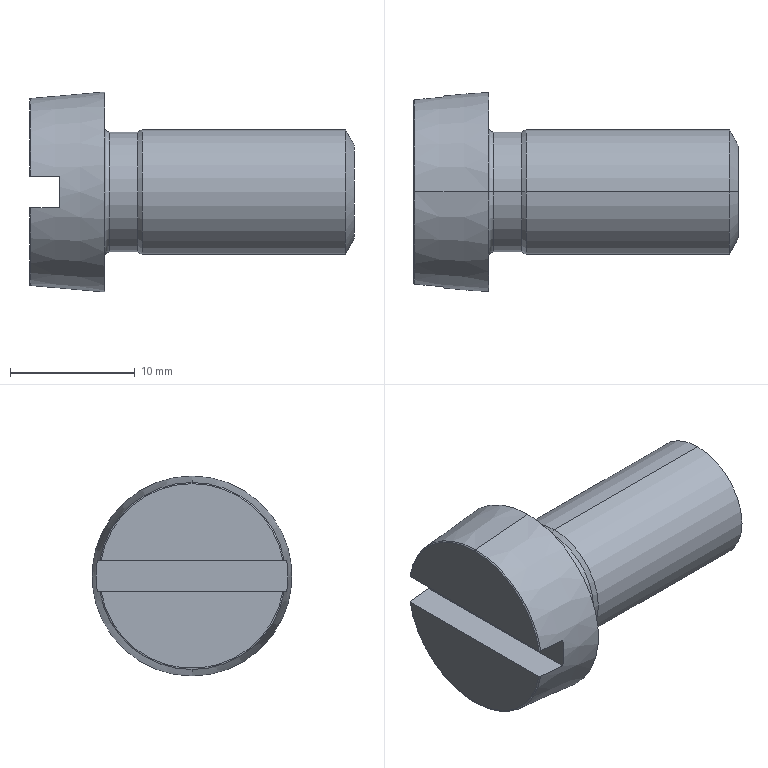Part | SolidWorks | features Cut 1, LPattern 1, RevCut 1, Revolution 1 | 1 solid | 22 faces | box 26 x 16 x 16 mm | volume 2579 mm3 | plane 7 | cone 6 | torus 5 | cylinder 4 | commonest cylinder face diameters 9.6 x2 10 x2
STEP:
#1=CARTESIAN_POINT('',(26.,0.,3.701));
#2=VERTEX_POINT('',#1);
#3=CARTESIAN_POINT('',(26.,0.,-3.701));
#4=VERTEX_POINT('',#3);
#5=CARTESIAN_POINT('',(26.,0.,0.));
#6=DIRECTION('',(-1.,0.,0.));
#7=DIRECTION('',(0.,0.,1.));
#8=AXIS2_PLACEMENT_3D('',#5,#6,#7);
#9=CIRCLE('',#8,3.701);
#10=EDGE_CURVE('',#2,#4,#9,.T.);
#11=ORIENTED_EDGE('',*,*,#10,.T.);
#12=CARTESIAN_POINT('',(25.25,0.,-5.));
#13=VERTEX_POINT('',#12);
#14=CARTESIAN_POINT('',(25.25,0.,-5.));
#15=DIRECTION('',(-0.5,0.,-0.866));
#16=VECTOR('',#15,1000.);
#17=LINE('',#14,#16);
#18=EDGE_CURVE('',#4,#13,#17,.T.);
#19=ORIENTED_EDGE('',*,*,#18,.T.);
#20=CARTESIAN_POINT('',(25.25,0.,5.));
#21=VERTEX_POINT('',#20);
#22=CARTESIAN_POINT('',(25.25,0.,0.));
#23=DIRECTION('',(-1.,0.,0.));
#24=DIRECTION('',(0.,0.,1.));
#25=AXIS2_PLACEMENT_3D('',#22,#23,#24);
#26=CIRCLE('',#25,5.);
#27=EDGE_CURVE('',#21,#13,#26,.T.);
#28=ORIENTED_EDGE('',*,*,#27,.F.);
#29=CARTESIAN_POINT('',(25.25,0.,5.));
#30=DIRECTION('',(-0.5,0.,0.866));
#31=VECTOR('',#30,1000.);
#32=LINE('',#29,#31);
#33=EDGE_CURVE('',#2,#21,#32,.T.);
#34=ORIENTED_EDGE('',*,*,#33,.F.);
#35=EDGE_LOOP('',(#11,#19,#28,#34));
#36=FACE_OUTER_BOUND('',#35,.T.);
#37=CARTESIAN_POINT('',(25.25,0.,0.));
#38=DIRECTION('',(-1.,0.,0.));
#39=DIRECTION('',(0.,0.,1.));
#40=AXIS2_PLACEMENT_3D('',#37,#38,#39);
#41=CONICAL_SURFACE('',#40,5.,1.047);
#42=ADVANCED_FACE('',(#36),#41,.T.);
#43=CARTESIAN_POINT('',(8.654,0.,4.8));
#44=VERTEX_POINT('',#43);
#45=CARTESIAN_POINT('',(8.654,0.,-4.8));
#46=VERTEX_POINT('',#45);
#47=CARTESIAN_POINT('',(8.654,0.,0.));
#48=DIRECTION('',(-1.,0.,0.));
#49=DIRECTION('',(0.,0.,1.));
#50=AXIS2_PLACEMENT_3D('',#47,#48,#49);
#51=CIRCLE('',#50,4.8);
#52=EDGE_CURVE('',#44,#46,#51,.T.);
#53=ORIENTED_EDGE('',*,*,#52,.F.);
#54=CARTESIAN_POINT('',(9.,0.,5.));
#55=VERTEX_POINT('',#54);
#56=CARTESIAN_POINT('',(9.,0.,5.));
#57=DIRECTION('',(0.866,0.,0.5));
#58=VECTOR('',#57,1000.);
#59=LINE('',#56,#58);
#60=EDGE_CURVE('',#44,#55,#59,.T.);
#61=ORIENTED_EDGE('',*,*,#60,.T.);
#62=CARTESIAN_POINT('',(9.,0.,-5.));
#63=VERTEX_POINT('',#62);
#64=CARTESIAN_POINT('',(9.,0.,0.));
#65=DIRECTION('',(-1.,0.,0.));
#66=DIRECTION('',(0.,0.,1.));
#67=AXIS2_PLACEMENT_3D('',#64,#65,#66);
#68=CIRCLE('',#67,5.);
#69=EDGE_CURVE('',#55,#63,#68,.T.);
#70=ORIENTED_EDGE('',*,*,#69,.T.);
#71=CARTESIAN_POINT('',(9.,0.,-5.));
#72=DIRECTION('',(0.866,0.,-0.5));
#73=VECTOR('',#72,1000.);
#74=LINE('',#71,#73);
#75=EDGE_CURVE('',#46,#63,#74,.T.);
#76=ORIENTED_EDGE('',*,*,#75,.F.);
#77=EDGE_LOOP('',(#53,#61,#70,#76));
#78=FACE_OUTER_BOUND('',#77,.T.);
#79=CARTESIAN_POINT('',(9.,0.,0.));
#80=DIRECTION('',(1.,0.,0.));
#81=DIRECTION('',(0.,0.,-1.));
#82=AXIS2_PLACEMENT_3D('',#79,#80,#81);
#83=CONICAL_SURFACE('',#82,5.,0.5236);
#84=ADVANCED_FACE('',(#78),#83,.T.);
#85=ORIENTED_EDGE('',*,*,#52,.T.);
#86=CARTESIAN_POINT('',(6.4,0.,-4.8));
#87=VERTEX_POINT('',#86);
#88=CARTESIAN_POINT('',(0.,0.,-4.8));
#89=DIRECTION('',(-1.,0.,0.));
#90=VECTOR('',#89,1000.);
#91=LINE('',#88,#90);
#92=EDGE_CURVE('',#46,#87,#91,.T.);
#93=ORIENTED_EDGE('',*,*,#92,.T.);
#94=CARTESIAN_POINT('',(6.4,0.,4.8));
#95=VERTEX_POINT('',#94);
#96=CARTESIAN_POINT('',(6.4,0.,0.));
#97=DIRECTION('',(-1.,0.,0.));
#98=DIRECTION('',(0.,0.,1.));
#99=AXIS2_PLACEMENT_3D('',#96,#97,#98);
#100=CIRCLE('',#99,4.8);
#101=EDGE_CURVE('',#95,#87,#100,.T.);
#102=ORIENTED_EDGE('',*,*,#101,.F.);
#103=CARTESIAN_POINT('',(0.,0.,4.8));
#104=DIRECTION('',(-1.,0.,0.));
#105=VECTOR('',#104,1000.);
#106=LINE('',#103,#105);
#107=EDGE_CURVE('',#44,#95,#106,.T.);
#108=ORIENTED_EDGE('',*,*,#107,.F.);
#109=EDGE_LOOP('',(#85,#93,#102,#108));
#110=FACE_OUTER_BOUND('',#109,.T.);
#111=CARTESIAN_POINT('',(0.,0.,0.));
#112=DIRECTION('',(-1.,0.,0.));
#113=DIRECTION('',(0.,0.,1.));
#114=AXIS2_PLACEMENT_3D('',#111,#112,#113);
#115=CYLINDRICAL_SURFACE('',#114,4.8);
#116=ADVANCED_FACE('',(#110),#115,.T.);
#117=CARTESIAN_POINT('',(6.,0.,-5.2));
#118=VERTEX_POINT('',#117);
#119=CARTESIAN_POINT('',(6.,0.,5.2));
#120=VERTEX_POINT('',#119);
#121=CARTESIAN_POINT('',(6.,0.,0.));
#122=DIRECTION('',(-1.,0.,0.));
#123=DIRECTION('',(0.,0.,1.));
#124=AXIS2_PLACEMENT_3D('',#121,#122,#123);
#125=CIRCLE('',#124,5.2);
#126=EDGE_CURVE('',#118,#120,#125,.T.);
#127=ORIENTED_EDGE('',*,*,#126,.F.);
#128=CARTESIAN_POINT('',(6.4,0.,-5.2));
#129=DIRECTION('',(0.,1.,0.));
#130=DIRECTION('',(0.,0.,1.));
#131=AXIS2_PLACEMENT_3D('',#128,#129,#130);
#132=CIRCLE('',#131,0.4);
#133=EDGE_CURVE('',#118,#87,#132,.T.);
#134=ORIENTED_EDGE('',*,*,#133,.T.);
#135=CARTESIAN_POINT('',(6.4,0.,0.));
#136=DIRECTION('',(-1.,0.,0.));
#137=DIRECTION('',(0.,0.,1.));
#138=AXIS2_PLACEMENT_3D('',#135,#136,#137);
#139=CIRCLE('',#138,4.8);
#140=EDGE_CURVE('',#87,#95,#139,.T.);
#141=ORIENTED_EDGE('',*,*,#140,.T.);
#142=CARTESIAN_POINT('',(6.4,0.,5.2));
#143=DIRECTION('',(0.,-1.,0.));
#144=DIRECTION('',(0.,0.,-1.));
#145=AXIS2_PLACEMENT_3D('',#142,#143,#144);
#146=CIRCLE('',#145,0.4);
#147=EDGE_CURVE('',#120,#95,#146,.T.);
#148=ORIENTED_EDGE('',*,*,#147,.F.);
#149=EDGE_LOOP('',(#127,#134,#141,#148));
#150=FACE_OUTER_BOUND('',#149,.T.);
#151=CARTESIAN_POINT('',(6.4,0.,0.));
#152=DIRECTION('',(-1.,0.,0.));
#153=DIRECTION('',(0.,0.,1.));
#154=AXIS2_PLACEMENT_3D('',#151,#152,#153);
#155=TOROIDAL_SURFACE('',#154,5.2,0.4);
#156=ADVANCED_FACE('',(#150),#155,.F.);
#157=CARTESIAN_POINT('',(0.09128,0.,7.483));
#158=VERTEX_POINT('',#157);
#159=CARTESIAN_POINT('',(0.09128,7.378,1.25));
#160=VERTEX_POINT('',#159);
#161=CARTESIAN_POINT('',(0.09128,0.,0.));
#162=DIRECTION('',(-1.,0.,0.));
#163=DIRECTION('',(0.,0.,1.));
#164=AXIS2_PLACEMENT_3D('',#161,#162,#163);
#165=CIRCLE('',#164,7.483);
#166=EDGE_CURVE('',#158,#160,#165,.T.);
#167=ORIENTED_EDGE('',*,*,#166,.F.);
#168=CARTESIAN_POINT('',(6.,0.,8.));
#169=VERTEX_POINT('',#168);
#170=CARTESIAN_POINT('',(6.,0.,8.));
#171=DIRECTION('',(0.9962,0.,0.08716));
#172=VECTOR('',#171,1000.);
#173=LINE('',#170,#172);
#174=EDGE_CURVE('',#158,#169,#173,.T.);
#175=ORIENTED_EDGE('',*,*,#174,.T.);
#176=CARTESIAN_POINT('',(6.,0.,-8.));
#177=VERTEX_POINT('',#176);
#178=CARTESIAN_POINT('',(6.,0.,0.));
#179=DIRECTION('',(-1.,0.,0.));
#180=DIRECTION('',(0.,0.,1.));
#181=AXIS2_PLACEMENT_3D('',#178,#179,#180);
#182=CIRCLE('',#181,8.);
#183=EDGE_CURVE('',#169,#177,#182,.T.);
#184=ORIENTED_EDGE('',*,*,#183,.T.);
#185=CARTESIAN_POINT('',(0.09128,0.,-7.483));
#186=VERTEX_POINT('',#185);
#187=CARTESIAN_POINT('',(6.,0.,-8.));
#188=DIRECTION('',(0.9962,0.,-0.08716));
#189=VECTOR('',#188,1000.);
#190=LINE('',#187,#189);
#191=EDGE_CURVE('',#186,#177,#190,.T.);
#192=ORIENTED_EDGE('',*,*,#191,.F.);
#193=CARTESIAN_POINT('',(0.09128,7.378,-1.25));
#194=VERTEX_POINT('',#193);
#195=CARTESIAN_POINT('',(0.09128,0.,0.));
#196=DIRECTION('',(-1.,0.,0.));
#197=DIRECTION('',(0.,0.,1.));
#198=AXIS2_PLACEMENT_3D('',#195,#196,#197);
#199=CIRCLE('',#198,7.483);
#200=EDGE_CURVE('',#194,#186,#199,.T.);
#201=ORIENTED_EDGE('',*,*,#200,.F.);
#202=CARTESIAN_POINT('',(2.4,7.583,-1.25));
#203=VERTEX_POINT('',#202);
#204=CARTESIAN_POINT('',(0.09128,7.378,-1.25));
#205=CARTESIAN_POINT('',(0.4301,7.408,-1.25));
#206=CARTESIAN_POINT('',(0.769,7.438,-1.25));
#207=CARTESIAN_POINT('',(1.108,7.468,-1.25));
#208=CARTESIAN_POINT('',(1.539,7.506,-1.25));
#209=CARTESIAN_POINT('',(1.969,7.545,-1.25));
#210=CARTESIAN_POINT('',(2.4,7.583,-1.25));
#211=B_SPLINE_CURVE_WITH_KNOTS('',3,(#204,#205,#206,#207,#208,#209,#210),.UNSPECIFIED.,.F.,.F.,(4,3,4),(0.01291,0.01393,0.01523),.UNSPECIFIED.);
#212=EDGE_CURVE('',#194,#203,#211,.T.);
#213=ORIENTED_EDGE('',*,*,#212,.T.);
#214=CARTESIAN_POINT('',(2.4,7.583,1.25));
#215=VERTEX_POINT('',#214);
#216=CARTESIAN_POINT('',(2.4,0.,0.));
#217=DIRECTION('',(-1.,0.,0.));
#218=DIRECTION('',(0.,-1.,0.));
#219=AXIS2_PLACEMENT_3D('',#216,#217,#218);
#220=CIRCLE('',#219,7.685);
#221=EDGE_CURVE('',#215,#203,#220,.T.);
#222=ORIENTED_EDGE('',*,*,#221,.F.);
#223=CARTESIAN_POINT('',(2.4,7.583,1.25));
#224=CARTESIAN_POINT('',(1.969,7.545,1.25));
#225=CARTESIAN_POINT('',(1.539,7.506,1.25));
#226=CARTESIAN_POINT('',(1.108,7.468,1.25));
#227=CARTESIAN_POINT('',(0.769,7.438,1.25));
#228=CARTESIAN_POINT('',(0.4301,7.408,1.25));
#229=CARTESIAN_POINT('',(0.09128,7.378,1.25));
#230=B_SPLINE_CURVE_WITH_KNOTS('',3,(#223,#224,#225,#226,#227,#228,#229),.UNSPECIFIED.,.F.,.F.,(4,3,4),(0.01263,0.01393,0.01495),.UNSPECIFIED.);
#231=EDGE_CURVE('',#215,#160,#230,.T.);
#232=ORIENTED_EDGE('',*,*,#231,.T.);
#233=EDGE_LOOP('',(#167,#175,#184,#192,#201,#213,#222,#232));
#234=FACE_OUTER_BOUND('',#233,.T.);
#235=CARTESIAN_POINT('',(6.,0.,0.));
#236=DIRECTION('',(1.,0.,0.));
#237=DIRECTION('',(0.,0.,-1.));
#238=AXIS2_PLACEMENT_3D('',#235,#236,#237);
#239=CONICAL_SURFACE('',#238,8.,0.08727);
#240=ADVANCED_FACE('',(#234),#239,.T.);
#241=CARTESIAN_POINT('',(0.09128,-7.378,1.25));
#242=VERTEX_POINT('',#241);
#243=CARTESIAN_POINT('',(0.09128,0.,0.));
#244=DIRECTION('',(-1.,0.,0.));
#245=DIRECTION('',(0.,0.,1.));
#246=AXIS2_PLACEMENT_3D('',#243,#244,#245);
#247=CIRCLE('',#246,7.483);
#248=EDGE_CURVE('',#242,#158,#247,.T.);
#249=ORIENTED_EDGE('',*,*,#248,.T.);
#250=CARTESIAN_POINT('',(0.,0.,7.383));
#251=VERTEX_POINT('',#250);
#252=CARTESIAN_POINT('',(0.1,0.,7.383));
#253=DIRECTION('',(0.,-1.,0.));
#254=DIRECTION('',(0.,0.,-1.));
#255=AXIS2_PLACEMENT_3D('',#252,#253,#254);
#256=CIRCLE('',#255,0.1);
#257=EDGE_CURVE('',#158,#251,#256,.T.);
#258=ORIENTED_EDGE('',*,*,#257,.T.);
#259=CARTESIAN_POINT('',(0.,-7.277,1.25));
#260=VERTEX_POINT('',#259);
#261=CARTESIAN_POINT('',(0.,0.,0.));
#262=DIRECTION('',(-1.,0.,0.));
#263=DIRECTION('',(0.,0.,1.));
#264=AXIS2_PLACEMENT_3D('',#261,#262,#263);
#265=CIRCLE('',#264,7.383);
#266=EDGE_CURVE('',#260,#251,#265,.T.);
#267=ORIENTED_EDGE('',*,*,#266,.F.);
#268=CARTESIAN_POINT('',(0.,-7.277,1.25));
#269=CARTESIAN_POINT('',(0.,-7.286,1.25));
#270=CARTESIAN_POINT('',(0.001125,-7.294,1.25));
#271=CARTESIAN_POINT('',(0.003323,-7.303,1.25));
#272=CARTESIAN_POINT('',(0.006228,-7.314,1.25));
#273=CARTESIAN_POINT('',(0.0111,-7.325,1.25));
#274=CARTESIAN_POINT('',(0.01756,-7.334,1.25));
#275=CARTESIAN_POINT('',(0.0217,-7.34,1.25));
#276=CARTESIAN_POINT('',(0.02655,-7.346,1.25));
#277=CARTESIAN_POINT('',(0.03193,-7.351,1.25));
#278=CARTESIAN_POINT('',(0.04004,-7.359,1.25));
#279=CARTESIAN_POINT('',(0.04957,-7.365,1.25));
#280=CARTESIAN_POINT('',(0.05975,-7.37,1.25));
#281=CARTESIAN_POINT('',(0.06967,-7.374,1.25));
#282=CARTESIAN_POINT('',(0.08047,-7.377,1.25));
#283=CARTESIAN_POINT('',(0.09128,-7.378,1.25));
#284=B_SPLINE_CURVE_WITH_KNOTS('',3,(#268,#269,#270,#271,#272,#273,#274,#275,#276,#277,#278,#279,#280,#281,#282,#283),.UNSPECIFIED.,.F.,.F.,(4,3,3,3,3,4),(0.0005472,0.0005733,0.0006079,0.0006299,0.0006633,0.0006959),.UNSPECIFIED.);
#285=EDGE_CURVE('',#260,#242,#284,.T.);
#286=ORIENTED_EDGE('',*,*,#285,.T.);
#287=EDGE_LOOP('',(#249,#258,#267,#286));
#288=FACE_OUTER_BOUND('',#287,.T.);
#289=CARTESIAN_POINT('',(0.1,0.,0.));
#290=DIRECTION('',(-1.,0.,0.));
#291=DIRECTION('',(0.,0.,1.));
#292=AXIS2_PLACEMENT_3D('',#289,#290,#291);
#293=TOROIDAL_SURFACE('',#292,7.383,0.1);
#294=ADVANCED_FACE('',(#288),#293,.T.);
#295=ORIENTED_EDGE('',*,*,#27,.T.);
#296=CARTESIAN_POINT('',(0.,0.,-5.));
#297=DIRECTION('',(-1.,0.,0.));
#298=VECTOR('',#297,1000.);
#299=LINE('',#296,#298);
#300=EDGE_CURVE('',#13,#63,#299,.T.);
#301=ORIENTED_EDGE('',*,*,#300,.T.);
#302=ORIENTED_EDGE('',*,*,#69,.F.);
#303=CARTESIAN_POINT('',(0.,0.,5.));
#304=DIRECTION('',(-1.,0.,0.));
#305=VECTOR('',#304,1000.);
#306=LINE('',#303,#305);
#307=EDGE_CURVE('',#21,#55,#306,.T.);
#308=ORIENTED_EDGE('',*,*,#307,.F.);
#309=EDGE_LOOP('',(#295,#301,#302,#308));
#310=FACE_OUTER_BOUND('',#309,.T.);
#311=CARTESIAN_POINT('',(0.,0.,0.));
#312=DIRECTION('',(-1.,0.,0.));
#313=DIRECTION('',(0.,0.,1.));
#314=AXIS2_PLACEMENT_3D('',#311,#312,#313);
#315=CYLINDRICAL_SURFACE('',#314,5.);
#316=ADVANCED_FACE('',(#310),#315,.T.);
#317=ORIENTED_EDGE('',*,*,#300,.F.);
#318=CARTESIAN_POINT('',(25.25,0.,0.));
#319=DIRECTION('',(-1.,0.,0.));
#320=DIRECTION('',(0.,0.,1.));
#321=AXIS2_PLACEMENT_3D('',#318,#319,#320);
#322=CIRCLE('',#321,5.);
#323=EDGE_CURVE('',#13,#21,#322,.T.);
#324=ORIENTED_EDGE('',*,*,#323,.T.);
#325=ORIENTED_EDGE('',*,*,#307,.T.);
#326=CARTESIAN_POINT('',(9.,0.,0.));
#327=DIRECTION('',(-1.,0.,0.));
#328=DIRECTION('',(0.,0.,1.));
#329=AXIS2_PLACEMENT_3D('',#326,#327,#328);
#330=CIRCLE('',#329,5.);
#331=EDGE_CURVE('',#63,#55,#330,.T.);
#332=ORIENTED_EDGE('',*,*,#331,.F.);
#333=EDGE_LOOP('',(#317,#324,#325,#332));
#334=FACE_OUTER_BOUND('',#333,.T.);
#335=CARTESIAN_POINT('',(0.,0.,0.));
#336=DIRECTION('',(-1.,0.,0.));
#337=DIRECTION('',(0.,0.,1.));
#338=AXIS2_PLACEMENT_3D('',#335,#336,#337);
#339=CYLINDRICAL_SURFACE('',#338,5.);
#340=ADVANCED_FACE('',(#334),#339,.T.);
#341=ORIENTED_EDGE('',*,*,#266,.T.);
#342=CARTESIAN_POINT('',(0.,7.277,1.25));
#343=VERTEX_POINT('',#342);
#344=CARTESIAN_POINT('',(0.,0.,0.));
#345=DIRECTION('',(-1.,0.,0.));
#346=DIRECTION('',(0.,0.,1.));
#347=AXIS2_PLACEMENT_3D('',#344,#345,#346);
#348=CIRCLE('',#347,7.383);
#349=EDGE_CURVE('',#251,#343,#348,.T.);
#350=ORIENTED_EDGE('',*,*,#349,.T.);
#351=CARTESIAN_POINT('',(0.,7.902,1.25));
#352=DIRECTION('',(0.,1.,0.));
#353=VECTOR('',#352,1000.);
#354=LINE('',#351,#353);
#355=EDGE_CURVE('',#260,#343,#354,.T.);
#356=ORIENTED_EDGE('',*,*,#355,.F.);
#357=EDGE_LOOP('',(#341,#350,#356));
#358=FACE_OUTER_BOUND('',#357,.T.);
#359=CARTESIAN_POINT('',(0.,0.,0.));
#360=DIRECTION('',(1.,0.,0.));
#361=DIRECTION('',(0.,0.,-1.));
#362=AXIS2_PLACEMENT_3D('',#359,#360,#361);
#363=PLANE('',#362);
#364=ADVANCED_FACE('',(#358),#363,.F.);
#365=ORIENTED_EDGE('',*,*,#257,.F.);
#366=ORIENTED_EDGE('',*,*,#166,.T.);
#367=CARTESIAN_POINT('',(0.09128,7.378,1.25));
#368=CARTESIAN_POINT('',(0.08575,7.377,1.25));
#369=CARTESIAN_POINT('',(0.08023,7.376,1.25));
#370=CARTESIAN_POINT('',(0.07485,7.375,1.25));
#371=CARTESIAN_POINT('',(0.06418,7.372,1.25));
#372=CARTESIAN_POINT('',(0.05384,7.368,1.25));
#373=CARTESIAN_POINT('',(0.04468,7.361,1.25));
#374=CARTESIAN_POINT('',(0.03547,7.355,1.25));
#375=CARTESIAN_POINT('',(0.02719,7.347,1.25));
#376=CARTESIAN_POINT('',(0.02051,7.338,1.25));
#377=CARTESIAN_POINT('',(0.01375,7.329,1.25));
#378=CARTESIAN_POINT('',(0.008429,7.319,1.25));
#379=CARTESIAN_POINT('',(0.00497,7.308,1.25));
#380=CARTESIAN_POINT('',(0.001695,7.298,1.25));
#381=CARTESIAN_POINT('',(0.,7.288,1.25));
#382=CARTESIAN_POINT('',(0.,7.277,1.25));
#383=B_SPLINE_CURVE_WITH_KNOTS('',3,(#367,#368,#369,#370,#371,#372,#373,#374,#375,#376,#377,#378,#379,#380,#381,#382),.UNSPECIFIED.,.F.,.F.,(4,3,3,3,3,4),(0.0003879,0.0004045,0.0004376,0.0004709,0.0005047,0.0005367),.UNSPECIFIED.);
#384=EDGE_CURVE('',#160,#343,#383,.T.);
#385=ORIENTED_EDGE('',*,*,#384,.T.);
#386=ORIENTED_EDGE('',*,*,#349,.F.);
#387=EDGE_LOOP('',(#365,#366,#385,#386));
#388=FACE_OUTER_BOUND('',#387,.T.);
#389=CARTESIAN_POINT('',(0.1,0.,0.));
#390=DIRECTION('',(-1.,0.,0.));
#391=DIRECTION('',(0.,0.,1.));
#392=AXIS2_PLACEMENT_3D('',#389,#390,#391);
#393=TOROIDAL_SURFACE('',#392,7.383,0.1);
#394=ADVANCED_FACE('',(#388),#393,.T.);
#395=CARTESIAN_POINT('',(0.,7.277,-1.25));
#396=VERTEX_POINT('',#395);
#397=CARTESIAN_POINT('',(0.,-7.277,-1.25));
#398=VERTEX_POINT('',#397);
#399=CARTESIAN_POINT('',(0.,0.,0.));
#400=DIRECTION('',(-1.,0.,0.));
#401=DIRECTION('',(0.,0.,1.));
#402=AXIS2_PLACEMENT_3D('',#399,#400,#401);
#403=CIRCLE('',#402,7.383);
#404=EDGE_CURVE('',#396,#398,#403,.T.);
#405=ORIENTED_EDGE('',*,*,#404,.T.);
#406=CARTESIAN_POINT('',(0.,7.902,-1.25));
#407=DIRECTION('',(0.,-1.,0.));
#408=VECTOR('',#407,1000.);
#409=LINE('',#406,#408);
#410=EDGE_CURVE('',#396,#398,#409,.T.);
#411=ORIENTED_EDGE('',*,*,#410,.F.);
#412=EDGE_LOOP('',(#405,#411));
#413=FACE_OUTER_BOUND('',#412,.T.);
#414=CARTESIAN_POINT('',(0.,0.,0.));
#415=DIRECTION('',(1.,0.,0.));
#416=DIRECTION('',(0.,0.,-1.));
#417=AXIS2_PLACEMENT_3D('',#414,#415,#416);
#418=PLANE('',#417);
#419=ADVANCED_FACE('',(#413),#418,.F.);
#420=ORIENTED_EDGE('',*,*,#200,.T.);
#421=CARTESIAN_POINT('',(0.09128,-7.378,-1.25));
#422=VERTEX_POINT('',#421);
#423=CARTESIAN_POINT('',(0.09128,0.,0.));
#424=DIRECTION('',(-1.,0.,0.));
#425=DIRECTION('',(0.,0.,1.));
#426=AXIS2_PLACEMENT_3D('',#423,#424,#425);
#427=CIRCLE('',#426,7.483);
#428=EDGE_CURVE('',#186,#422,#427,.T.);
#429=ORIENTED_EDGE('',*,*,#428,.T.);
#430=CARTESIAN_POINT('',(0.09128,-7.378,-1.25));
#431=CARTESIAN_POINT('',(0.08699,-7.378,-1.25));
#432=CARTESIAN_POINT('',(0.08271,-7.377,-1.25));
#433=CARTESIAN_POINT('',(0.07851,-7.376,-1.25));
#434=CARTESIAN_POINT('',(0.06773,-7.374,-1.25));
#435=CARTESIAN_POINT('',(0.05723,-7.369,-1.25));
#436=CARTESIAN_POINT('',(0.04784,-7.363,-1.25));
#437=CARTESIAN_POINT('',(0.04216,-7.36,-1.25));
#438=CARTESIAN_POINT('',(0.0368,-7.356,-1.25));
#439=CARTESIAN_POINT('',(0.03193,-7.351,-1.25));
#440=CARTESIAN_POINT('',(0.02366,-7.343,-1.25));
#441=CARTESIAN_POINT('',(0.01663,-7.334,-1.25));
#442=CARTESIAN_POINT('',(0.01141,-7.324,-1.25));
#443=CARTESIAN_POINT('',(0.006197,-7.314,-1.25));
#444=CARTESIAN_POINT('',(0.002648,-7.303,-1.25));
#445=CARTESIAN_POINT('',(0.001037,-7.291,-1.25));
#446=CARTESIAN_POINT('',(0.0003474,-7.287,-1.25));
#447=CARTESIAN_POINT('',(0.,-7.282,-1.25));
#448=CARTESIAN_POINT('',(0.,-7.277,-1.25));
#449=B_SPLINE_CURVE_WITH_KNOTS('',3,(#430,#431,#432,#433,#434,#435,#436,#437,#438,#439,#440,#441,#442,#443,#444,#445,#446,#447,#448),.UNSPECIFIED.,.F.,.F.,(4,3,3,3,3,3,4),(0.0005639,0.0005767,0.0006098,0.0006297,0.0006638,0.0006979,0.0007125),.UNSPECIFIED.);
#450=EDGE_CURVE('',#422,#398,#449,.T.);
#451=ORIENTED_EDGE('',*,*,#450,.T.);
#452=ORIENTED_EDGE('',*,*,#404,.F.);
#453=CARTESIAN_POINT('',(0.,7.277,-1.25));
#454=CARTESIAN_POINT('',(0.,7.28,-1.25));
#455=CARTESIAN_POINT('',(0.0001312,7.283,-1.25));
#456=CARTESIAN_POINT('',(0.0003928,7.286,-1.25));
#457=CARTESIAN_POINT('',(0.001398,7.297,-1.25));
#458=CARTESIAN_POINT('',(0.004397,7.309,-1.25));
#459=CARTESIAN_POINT('',(0.009153,7.319,-1.25));
#460=CARTESIAN_POINT('',(0.0139,7.33,-1.25));
#461=CARTESIAN_POINT('',(0.02052,7.34,-1.25));
#462=CARTESIAN_POINT('',(0.0285,7.348,-1.25));
#463=CARTESIAN_POINT('',(0.03638,7.356,-1.25));
#464=CARTESIAN_POINT('',(0.0458,7.363,-1.25));
#465=CARTESIAN_POINT('',(0.05598,7.368,-1.25));
#466=CARTESIAN_POINT('',(0.06601,7.373,-1.25));
#467=CARTESIAN_POINT('',(0.07705,7.376,-1.25));
#468=CARTESIAN_POINT('',(0.08817,7.378,-1.25));
#469=CARTESIAN_POINT('',(0.08921,7.378,-1.25));
#470=CARTESIAN_POINT('',(0.09025,7.378,-1.25));
#471=CARTESIAN_POINT('',(0.09128,7.378,-1.25));
#472=B_SPLINE_CURVE_WITH_KNOTS('',3,(#453,#454,#455,#456,#457,#458,#459,#460,#461,#462,#463,#464,#465,#466,#467,#468,#469,#470,#471),.UNSPECIFIED.,.F.,.F.,(4,3,3,3,3,3,4),(0.00009337,0.0001023,0.0001368,0.0001713,0.0002054,0.000239,0.0002421),.UNSPECIFIED.);
#473=EDGE_CURVE('',#396,#194,#472,.T.);
#474=ORIENTED_EDGE('',*,*,#473,.T.);
#475=EDGE_LOOP('',(#420,#429,#451,#452,#474));
#476=FACE_OUTER_BOUND('',#475,.T.);
#477=CARTESIAN_POINT('',(0.1,0.,0.));
#478=DIRECTION('',(-1.,0.,0.));
#479=DIRECTION('',(0.,0.,1.));
#480=AXIS2_PLACEMENT_3D('',#477,#478,#479);
#481=TOROIDAL_SURFACE('',#480,7.383,0.1);
#482=ADVANCED_FACE('',(#476),#481,.T.);
#483=ORIENTED_EDGE('',*,*,#174,.F.);
#484=ORIENTED_EDGE('',*,*,#248,.F.);
#485=CARTESIAN_POINT('',(2.4,-7.583,1.25));
#486=VERTEX_POINT('',#485);
#487=CARTESIAN_POINT('',(0.09128,-7.378,1.25));
#488=CARTESIAN_POINT('',(0.4301,-7.408,1.25));
#489=CARTESIAN_POINT('',(0.769,-7.438,1.25));
#490=CARTESIAN_POINT('',(1.108,-7.468,1.25));
#491=CARTESIAN_POINT('',(1.539,-7.506,1.25));
#492=CARTESIAN_POINT('',(1.969,-7.545,1.25));
#493=CARTESIAN_POINT('',(2.4,-7.583,1.25));
#494=B_SPLINE_CURVE_WITH_KNOTS('',3,(#487,#488,#489,#490,#491,#492,#493),.UNSPECIFIED.,.F.,.F.,(4,3,4),(0.01291,0.01393,0.01523),.UNSPECIFIED.);
#495=EDGE_CURVE('',#242,#486,#494,.T.);
#496=ORIENTED_EDGE('',*,*,#495,.T.);
#497=CARTESIAN_POINT('',(2.4,-7.583,-1.25));
#498=VERTEX_POINT('',#497);
#499=CARTESIAN_POINT('',(2.4,0.,0.));
#500=DIRECTION('',(-1.,0.,0.));
#501=DIRECTION('',(0.,-1.,0.));
#502=AXIS2_PLACEMENT_3D('',#499,#500,#501);
#503=CIRCLE('',#502,7.685);
#504=EDGE_CURVE('',#498,#486,#503,.T.);
#505=ORIENTED_EDGE('',*,*,#504,.F.);
#506=CARTESIAN_POINT('',(2.4,-7.583,-1.25));
#507=CARTESIAN_POINT('',(1.969,-7.545,-1.25));
#508=CARTESIAN_POINT('',(1.539,-7.506,-1.25));
#509=CARTESIAN_POINT('',(1.108,-7.468,-1.25));
#510=CARTESIAN_POINT('',(0.769,-7.438,-1.25));
#511=CARTESIAN_POINT('',(0.4301,-7.408,-1.25));
#512=CARTESIAN_POINT('',(0.09128,-7.378,-1.25));
#513=B_SPLINE_CURVE_WITH_KNOTS('',3,(#506,#507,#508,#509,#510,#511,#512),.UNSPECIFIED.,.F.,.F.,(4,3,4),(0.01263,0.01393,0.01495),.UNSPECIFIED.);
#514=EDGE_CURVE('',#498,#422,#513,.T.);
#515=ORIENTED_EDGE('',*,*,#514,.T.);
#516=ORIENTED_EDGE('',*,*,#428,.F.);
#517=ORIENTED_EDGE('',*,*,#191,.T.);
#518=CARTESIAN_POINT('',(6.,0.,0.));
#519=DIRECTION('',(-1.,0.,0.));
#520=DIRECTION('',(0.,0.,1.));
#521=AXIS2_PLACEMENT_3D('',#518,#519,#520);
#522=CIRCLE('',#521,8.);
#523=EDGE_CURVE('',#177,#169,#522,.T.);
#524=ORIENTED_EDGE('',*,*,#523,.T.);
#525=EDGE_LOOP('',(#483,#484,#496,#505,#515,#516,#517,#524));
#526=FACE_OUTER_BOUND('',#525,.T.);
#527=CARTESIAN_POINT('',(6.,0.,0.));
#528=DIRECTION('',(1.,0.,0.));
#529=DIRECTION('',(0.,0.,-1.));
#530=AXIS2_PLACEMENT_3D('',#527,#528,#529);
#531=CONICAL_SURFACE('',#530,8.,0.08727);
#532=ADVANCED_FACE('',(#526),#531,.T.);
#533=ORIENTED_EDGE('',*,*,#523,.F.);
#534=ORIENTED_EDGE('',*,*,#183,.F.);
#535=EDGE_LOOP('',(#533,#534));
#536=FACE_OUTER_BOUND('',#535,.T.);
#537=CARTESIAN_POINT('',(6.,0.,0.));
#538=DIRECTION('',(-1.,0.,0.));
#539=DIRECTION('',(0.,0.,1.));
#540=AXIS2_PLACEMENT_3D('',#537,#538,#539);
#541=CIRCLE('',#540,5.2);
#542=EDGE_CURVE('',#120,#118,#541,.T.);
#543=ORIENTED_EDGE('',*,*,#542,.T.);
#544=ORIENTED_EDGE('',*,*,#126,.T.);
#545=EDGE_LOOP('',(#543,#544));
#546=FACE_BOUND('',#545,.T.);
#547=CARTESIAN_POINT('',(6.,8.,0.));
#548=DIRECTION('',(-1.,0.,0.));
#549=DIRECTION('',(0.,0.,1.));
#550=AXIS2_PLACEMENT_3D('',#547,#548,#549);
#551=PLANE('',#550);
#552=ADVANCED_FACE('',(#536,#546),#551,.F.);
#553=ORIENTED_EDGE('',*,*,#133,.F.);
#554=ORIENTED_EDGE('',*,*,#542,.F.);
#555=ORIENTED_EDGE('',*,*,#147,.T.);
#556=ORIENTED_EDGE('',*,*,#101,.T.);
#557=EDGE_LOOP('',(#553,#554,#555,#556));
#558=FACE_OUTER_BOUND('',#557,.T.);
#559=CARTESIAN_POINT('',(6.4,0.,0.));
#560=DIRECTION('',(-1.,0.,0.));
#561=DIRECTION('',(0.,0.,1.));
#562=AXIS2_PLACEMENT_3D('',#559,#560,#561);
#563=TOROIDAL_SURFACE('',#562,5.2,0.4);
#564=ADVANCED_FACE('',(#558),#563,.F.);
#565=ORIENTED_EDGE('',*,*,#92,.F.);
#566=CARTESIAN_POINT('',(8.654,0.,0.));
#567=DIRECTION('',(-1.,0.,0.));
#568=DIRECTION('',(0.,0.,1.));
#569=AXIS2_PLACEMENT_3D('',#566,#567,#568);
#570=CIRCLE('',#569,4.8);
#571=EDGE_CURVE('',#46,#44,#570,.T.);
#572=ORIENTED_EDGE('',*,*,#571,.T.);
#573=ORIENTED_EDGE('',*,*,#107,.T.);
#574=ORIENTED_EDGE('',*,*,#140,.F.);
#575=EDGE_LOOP('',(#565,#572,#573,#574));
#576=FACE_OUTER_BOUND('',#575,.T.);
#577=CARTESIAN_POINT('',(0.,0.,0.));
#578=DIRECTION('',(-1.,0.,0.));
#579=DIRECTION('',(0.,0.,1.));
#580=AXIS2_PLACEMENT_3D('',#577,#578,#579);
#581=CYLINDRICAL_SURFACE('',#580,4.8);
#582=ADVANCED_FACE('',(#576),#581,.T.);
#583=ORIENTED_EDGE('',*,*,#60,.F.);
#584=ORIENTED_EDGE('',*,*,#571,.F.);
#585=ORIENTED_EDGE('',*,*,#75,.T.);
#586=ORIENTED_EDGE('',*,*,#331,.T.);
#587=EDGE_LOOP('',(#583,#584,#585,#586));
#588=FACE_OUTER_BOUND('',#587,.T.);
#589=CARTESIAN_POINT('',(9.,0.,0.));
#590=DIRECTION('',(1.,0.,0.));
#591=DIRECTION('',(0.,0.,-1.));
#592=AXIS2_PLACEMENT_3D('',#589,#590,#591);
#593=CONICAL_SURFACE('',#592,5.,0.5236);
#594=ADVANCED_FACE('',(#588),#593,.T.);
#595=ORIENTED_EDGE('',*,*,#355,.T.);
#596=ORIENTED_EDGE('',*,*,#384,.F.);
#597=ORIENTED_EDGE('',*,*,#231,.F.);
#598=CARTESIAN_POINT('',(2.4,7.902,1.25));
#599=DIRECTION('',(0.,1.,0.));
#600=VECTOR('',#599,1000.);
#601=LINE('',#598,#600);
#602=EDGE_CURVE('',#486,#215,#601,.T.);
#603=ORIENTED_EDGE('',*,*,#602,.F.);
#604=ORIENTED_EDGE('',*,*,#495,.F.);
#605=ORIENTED_EDGE('',*,*,#285,.F.);
#606=EDGE_LOOP('',(#595,#596,#597,#603,#604,#605));
#607=FACE_OUTER_BOUND('',#606,.T.);
#608=CARTESIAN_POINT('',(2.4,7.902,1.25));
#609=DIRECTION('',(0.,0.,1.));
#610=DIRECTION('',(0.,-1.,0.));
#611=AXIS2_PLACEMENT_3D('',#608,#609,#610);
#612=PLANE('',#611);
#613=ADVANCED_FACE('',(#607),#612,.F.);
#614=ORIENTED_EDGE('',*,*,#514,.F.);
#615=CARTESIAN_POINT('',(2.4,7.902,-1.25));
#616=DIRECTION('',(0.,-1.,0.));
#617=VECTOR('',#616,1000.);
#618=LINE('',#615,#617);
#619=EDGE_CURVE('',#203,#498,#618,.T.);
#620=ORIENTED_EDGE('',*,*,#619,.F.);
#621=ORIENTED_EDGE('',*,*,#212,.F.);
#622=ORIENTED_EDGE('',*,*,#473,.F.);
#623=ORIENTED_EDGE('',*,*,#410,.T.);
#624=ORIENTED_EDGE('',*,*,#450,.F.);
#625=EDGE_LOOP('',(#614,#620,#621,#622,#623,#624));
#626=FACE_OUTER_BOUND('',#625,.T.);
#627=CARTESIAN_POINT('',(2.4,7.902,-1.25));
#628=DIRECTION('',(0.,0.,-1.));
#629=DIRECTION('',(-1.,0.,0.));
#630=AXIS2_PLACEMENT_3D('',#627,#628,#629);
#631=PLANE('',#630);
#632=ADVANCED_FACE('',(#626),#631,.F.);
#633=ORIENTED_EDGE('',*,*,#221,.T.);
#634=ORIENTED_EDGE('',*,*,#619,.T.);
#635=ORIENTED_EDGE('',*,*,#504,.T.);
#636=ORIENTED_EDGE('',*,*,#602,.T.);
#637=EDGE_LOOP('',(#633,#634,#635,#636));
#638=FACE_OUTER_BOUND('',#637,.T.);
#639=CARTESIAN_POINT('',(2.4,0.,0.));
#640=DIRECTION('',(-1.,0.,0.));
#641=DIRECTION('',(0.,-1.,0.));
#642=AXIS2_PLACEMENT_3D('',#639,#640,#641);
#643=PLANE('',#642);
#644=ADVANCED_FACE('',(#638),#643,.T.);
#645=ORIENTED_EDGE('',*,*,#18,.F.);
#646=CARTESIAN_POINT('',(26.,0.,0.));
#647=DIRECTION('',(-1.,0.,0.));
#648=DIRECTION('',(0.,0.,1.));
#649=AXIS2_PLACEMENT_3D('',#646,#647,#648);
#650=CIRCLE('',#649,3.701);
#651=EDGE_CURVE('',#4,#2,#650,.T.);
#652=ORIENTED_EDGE('',*,*,#651,.T.);
#653=ORIENTED_EDGE('',*,*,#33,.T.);
#654=ORIENTED_EDGE('',*,*,#323,.F.);
#655=EDGE_LOOP('',(#645,#652,#653,#654));
#656=FACE_OUTER_BOUND('',#655,.T.);
#657=CARTESIAN_POINT('',(25.25,0.,0.));
#658=DIRECTION('',(-1.,0.,0.));
#659=DIRECTION('',(0.,0.,1.));
#660=AXIS2_PLACEMENT_3D('',#657,#658,#659);
#661=CONICAL_SURFACE('',#660,5.,1.047);
#662=ADVANCED_FACE('',(#656),#661,.T.);
#663=ORIENTED_EDGE('',*,*,#10,.F.);
#664=ORIENTED_EDGE('',*,*,#651,.F.);
#665=EDGE_LOOP('',(#663,#664));
#666=FACE_OUTER_BOUND('',#665,.T.);
#667=CARTESIAN_POINT('',(26.,5.,0.));
#668=DIRECTION('',(-1.,0.,0.));
#669=DIRECTION('',(0.,0.,1.));
#670=AXIS2_PLACEMENT_3D('',#667,#668,#669);
#671=PLANE('',#670);
#672=ADVANCED_FACE('',(#666),#671,.F.);
#673=CLOSED_SHELL('',(#42,#84,#116,#156,#240,#294,#316,#340,#364,#394,#419,#482,#532,#552,#564,#582,#594,#613,#632,#644,#662,#672));
#674=MANIFOLD_SOLID_BREP('',#673);
#675=CARTESIAN_POINT('',(0.,0.,0.));
#676=DIRECTION('',(0.,0.,1.));
#677=DIRECTION('',(1.,0.,0.));
#678=AXIS2_PLACEMENT_3D('',#675,#676,#677);
#679=(LENGTH_UNIT()NAMED_UNIT(*)SI_UNIT(.MILLI.,.METRE.));
#680=UNCERTAINTY_MEASURE_WITH_UNIT(LENGTH_MEASURE(0.00001),#679,'','');
#681=(NAMED_UNIT(*)PLANE_ANGLE_UNIT()SI_UNIT($,.RADIAN.));
#682=(NAMED_UNIT(*)SI_UNIT($,.STERADIAN.)SOLID_ANGLE_UNIT());
#683=(GEOMETRIC_REPRESENTATION_CONTEXT(3)GLOBAL_UNCERTAINTY_ASSIGNED_CONTEXT((#680))GLOBAL_UNIT_ASSIGNED_CONTEXT((#679,#681,#682))REPRESENTATION_CONTEXT('',''));
#684=ADVANCED_BREP_SHAPE_REPRESENTATION('',(#674,#678),#683);